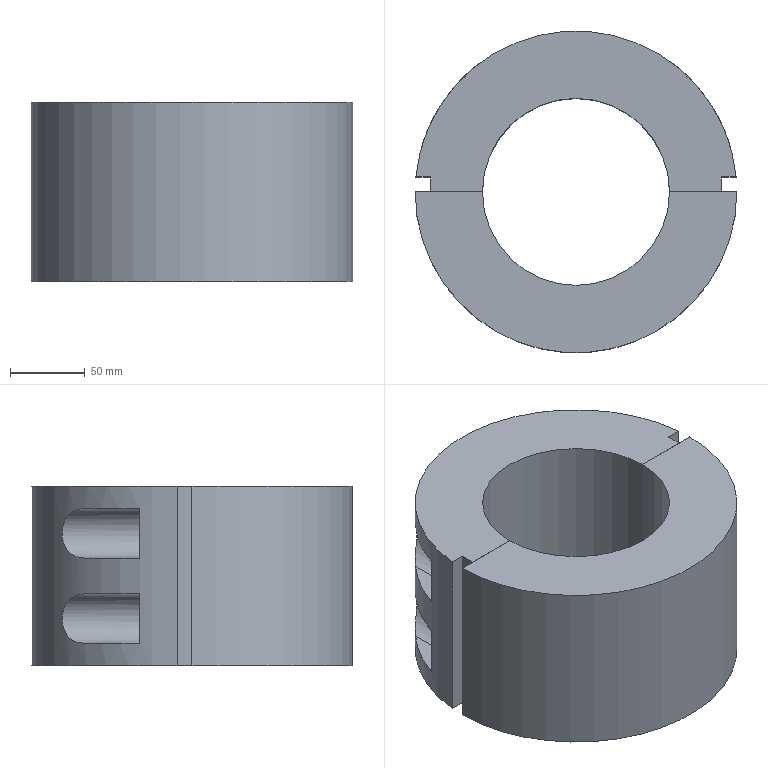Part | 2 solids | 44 faces | box 215 x 215 x 120 mm | volume 2640481 mm3 | plane 28 | cylinder 16 | commonest cylinder face diameters 17.5 x4 21.5 x4 33 x4 125 x2 215 x2
STEP:
#1=CARTESIAN_POINT('',(-80.,-35.,-79.75));
#2=VERTEX_POINT('',#1);
#3=CARTESIAN_POINT('',(-80.,-35.,-88.5));
#4=DIRECTION('',(0.,-1.,0.));
#5=DIRECTION('',(0.,0.,1.));
#6=AXIS2_PLACEMENT_3D('',#3,#4,#5);
#7=CIRCLE('',#6,8.75);
#8=EDGE_CURVE('',#2,#2,#7,.T.);
#9=ORIENTED_EDGE('',*,*,#8,.F.);
#10=EDGE_LOOP('',(#9));
#11=FACE_BOUND('',#10,.T.);
#12=CARTESIAN_POINT('',(-80.,-35.,-88.5));
#13=DIRECTION('',(0.,1.,0.));
#14=DIRECTION('',(0.,0.,1.));
#15=AXIS2_PLACEMENT_3D('',#12,#13,#14);
#16=PLANE('',#15);
#17=ADVANCED_FACE('',(#11),#16,.T.);
#18=ORIENTED_EDGE('',*,*,#8,.T.);
#19=EDGE_LOOP('',(#18));
#20=FACE_BOUND('',#19,.T.);
#21=CARTESIAN_POINT('',(-80.,0.,-79.75));
#22=VERTEX_POINT('',#21);
#23=CARTESIAN_POINT('',(-80.,0.,-88.5));
#24=DIRECTION('',(0.,-1.,0.));
#25=DIRECTION('',(0.,0.,1.));
#26=AXIS2_PLACEMENT_3D('',#23,#24,#25);
#27=CIRCLE('',#26,8.75);
#28=EDGE_CURVE('',#22,#22,#27,.T.);
#29=ORIENTED_EDGE('',*,*,#28,.F.);
#30=EDGE_LOOP('',(#29));
#31=FACE_BOUND('',#30,.T.);
#32=CARTESIAN_POINT('',(-80.,-35.,-88.5));
#33=DIRECTION('',(0.,1.,0.));
#34=DIRECTION('',(0.,0.,1.));
#35=AXIS2_PLACEMENT_3D('',#32,#33,#34);
#36=CYLINDRICAL_SURFACE('',#35,8.75);
#37=ADVANCED_FACE('',(#20,#31),#36,.F.);
#38=CARTESIAN_POINT('',(-80.,-35.,-40.25));
#39=VERTEX_POINT('',#38);
#40=CARTESIAN_POINT('',(-80.,-35.,-31.5));
#41=DIRECTION('',(0.,1.,0.));
#42=DIRECTION('',(0.,0.,-1.));
#43=AXIS2_PLACEMENT_3D('',#40,#41,#42);
#44=CIRCLE('',#43,8.75);
#45=EDGE_CURVE('',#39,#39,#44,.T.);
#46=ORIENTED_EDGE('',*,*,#45,.T.);
#47=EDGE_LOOP('',(#46));
#48=FACE_BOUND('',#47,.T.);
#49=CARTESIAN_POINT('',(-80.,-35.,-31.5));
#50=DIRECTION('',(0.,-1.,0.));
#51=DIRECTION('',(0.,0.,-1.));
#52=AXIS2_PLACEMENT_3D('',#49,#50,#51);
#53=PLANE('',#52);
#54=ADVANCED_FACE('',(#48),#53,.F.);
#55=ORIENTED_EDGE('',*,*,#45,.F.);
#56=EDGE_LOOP('',(#55));
#57=FACE_BOUND('',#56,.T.);
#58=CARTESIAN_POINT('',(-80.,0.,-22.75));
#59=VERTEX_POINT('',#58);
#60=CARTESIAN_POINT('',(-80.,0.,-31.5));
#61=DIRECTION('',(0.,-1.,0.));
#62=DIRECTION('',(0.,0.,1.));
#63=AXIS2_PLACEMENT_3D('',#60,#61,#62);
#64=CIRCLE('',#63,8.75);
#65=EDGE_CURVE('',#59,#59,#64,.T.);
#66=ORIENTED_EDGE('',*,*,#65,.F.);
#67=EDGE_LOOP('',(#66));
#68=FACE_BOUND('',#67,.T.);
#69=CARTESIAN_POINT('',(-80.,-35.,-31.5));
#70=DIRECTION('',(0.,1.,0.));
#71=DIRECTION('',(0.,0.,1.));
#72=AXIS2_PLACEMENT_3D('',#69,#70,#71);
#73=CYLINDRICAL_SURFACE('',#72,8.75);
#74=ADVANCED_FACE('',(#57,#68),#73,.F.);
#75=CARTESIAN_POINT('',(80.,-35.,-79.75));
#76=VERTEX_POINT('',#75);
#77=CARTESIAN_POINT('',(80.,-35.,-88.5));
#78=DIRECTION('',(0.,1.,0.));
#79=DIRECTION('',(0.,0.,1.));
#80=AXIS2_PLACEMENT_3D('',#77,#78,#79);
#81=CIRCLE('',#80,8.75);
#82=EDGE_CURVE('',#76,#76,#81,.F.);
#83=ORIENTED_EDGE('',*,*,#82,.F.);
#84=EDGE_LOOP('',(#83));
#85=FACE_BOUND('',#84,.T.);
#86=CARTESIAN_POINT('',(80.,-35.,-88.5));
#87=DIRECTION('',(0.,1.,0.));
#88=DIRECTION('',(0.,0.,1.));
#89=AXIS2_PLACEMENT_3D('',#86,#87,#88);
#90=PLANE('',#89);
#91=ADVANCED_FACE('',(#85),#90,.T.);
#92=CARTESIAN_POINT('',(80.,-35.,-40.25));
#93=VERTEX_POINT('',#92);
#94=CARTESIAN_POINT('',(80.,-35.,-31.5));
#95=DIRECTION('',(0.,-1.,0.));
#96=DIRECTION('',(0.,0.,-1.));
#97=AXIS2_PLACEMENT_3D('',#94,#95,#96);
#98=CIRCLE('',#97,8.75);
#99=EDGE_CURVE('',#93,#93,#98,.F.);
#100=ORIENTED_EDGE('',*,*,#99,.T.);
#101=EDGE_LOOP('',(#100));
#102=FACE_BOUND('',#101,.T.);
#103=CARTESIAN_POINT('',(80.,-35.,-31.5));
#104=DIRECTION('',(0.,-1.,0.));
#105=DIRECTION('',(0.,0.,-1.));
#106=AXIS2_PLACEMENT_3D('',#103,#104,#105);
#107=PLANE('',#106);
#108=ADVANCED_FACE('',(#102),#107,.F.);
#109=ORIENTED_EDGE('',*,*,#82,.T.);
#110=EDGE_LOOP('',(#109));
#111=FACE_BOUND('',#110,.T.);
#112=CARTESIAN_POINT('',(80.,0.,-79.75));
#113=VERTEX_POINT('',#112);
#114=CARTESIAN_POINT('',(80.,0.,-88.5));
#115=DIRECTION('',(0.,1.,0.));
#116=DIRECTION('',(0.,0.,1.));
#117=AXIS2_PLACEMENT_3D('',#114,#115,#116);
#118=CIRCLE('',#117,8.75);
#119=EDGE_CURVE('',#113,#113,#118,.T.);
#120=ORIENTED_EDGE('',*,*,#119,.T.);
#121=EDGE_LOOP('',(#120));
#122=FACE_BOUND('',#121,.T.);
#123=CARTESIAN_POINT('',(80.,-35.,-88.5));
#124=DIRECTION('',(0.,1.,0.));
#125=DIRECTION('',(0.,0.,1.));
#126=AXIS2_PLACEMENT_3D('',#123,#124,#125);
#127=CYLINDRICAL_SURFACE('',#126,8.75);
#128=ADVANCED_FACE('',(#111,#122),#127,.F.);
#129=ORIENTED_EDGE('',*,*,#99,.F.);
#130=EDGE_LOOP('',(#129));
#131=FACE_BOUND('',#130,.T.);
#132=CARTESIAN_POINT('',(80.,0.,-22.75));
#133=VERTEX_POINT('',#132);
#134=CARTESIAN_POINT('',(80.,0.,-31.5));
#135=DIRECTION('',(0.,1.,0.));
#136=DIRECTION('',(0.,0.,1.));
#137=AXIS2_PLACEMENT_3D('',#134,#135,#136);
#138=CIRCLE('',#137,8.75);
#139=EDGE_CURVE('',#133,#133,#138,.F.);
#140=ORIENTED_EDGE('',*,*,#139,.F.);
#141=EDGE_LOOP('',(#140));
#142=FACE_BOUND('',#141,.T.);
#143=CARTESIAN_POINT('',(80.,-35.,-31.5));
#144=DIRECTION('',(0.,1.,0.));
#145=DIRECTION('',(0.,0.,1.));
#146=AXIS2_PLACEMENT_3D('',#143,#144,#145);
#147=CYLINDRICAL_SURFACE('',#146,8.75);
#148=ADVANCED_FACE('',(#131,#142),#147,.F.);
#149=ORIENTED_EDGE('',*,*,#139,.T.);
#150=EDGE_LOOP('',(#149));
#151=FACE_BOUND('',#150,.T.);
#152=CARTESIAN_POINT('',(107.5,0.,0.));
#153=VERTEX_POINT('',#152);
#154=CARTESIAN_POINT('',(62.5,0.,0.));
#155=VERTEX_POINT('',#154);
#156=CARTESIAN_POINT('',(107.5,0.,0.));
#157=DIRECTION('',(-1.,0.,0.));
#158=VECTOR('',#157,1000.);
#159=LINE('',#156,#158);
#160=EDGE_CURVE('',#153,#155,#159,.T.);
#161=ORIENTED_EDGE('',*,*,#160,.F.);
#162=CARTESIAN_POINT('',(107.5,0.,-120.));
#163=VERTEX_POINT('',#162);
#164=CARTESIAN_POINT('',(107.5,0.,-120.));
#165=DIRECTION('',(0.,0.,1.));
#166=VECTOR('',#165,1000.);
#167=LINE('',#164,#166);
#168=EDGE_CURVE('',#163,#153,#167,.T.);
#169=ORIENTED_EDGE('',*,*,#168,.F.);
#170=CARTESIAN_POINT('',(62.5,0.,-120.));
#171=VERTEX_POINT('',#170);
#172=CARTESIAN_POINT('',(107.5,0.,-120.));
#173=DIRECTION('',(-1.,0.,0.));
#174=VECTOR('',#173,1000.);
#175=LINE('',#172,#174);
#176=EDGE_CURVE('',#163,#171,#175,.T.);
#177=ORIENTED_EDGE('',*,*,#176,.T.);
#178=CARTESIAN_POINT('',(62.5,0.,-120.));
#179=DIRECTION('',(0.,0.,1.));
#180=VECTOR('',#179,1000.);
#181=LINE('',#178,#180);
#182=EDGE_CURVE('',#171,#155,#181,.T.);
#183=ORIENTED_EDGE('',*,*,#182,.T.);
#184=EDGE_LOOP('',(#161,#169,#177,#183));
#185=FACE_BOUND('',#184,.T.);
#186=ORIENTED_EDGE('',*,*,#119,.F.);
#187=EDGE_LOOP('',(#186));
#188=FACE_BOUND('',#187,.T.);
#189=CARTESIAN_POINT('',(107.5,0.,-120.));
#190=DIRECTION('',(0.,1.,0.));
#191=DIRECTION('',(0.,0.,1.));
#192=AXIS2_PLACEMENT_3D('',#189,#190,#191);
#193=PLANE('',#192);
#194=ADVANCED_FACE('',(#151,#185,#188),#193,.T.);
#195=CARTESIAN_POINT('',(-107.5,0.,0.));
#196=VERTEX_POINT('',#195);
#197=CARTESIAN_POINT('',(0.,0.,0.));
#198=DIRECTION('',(0.,0.,1.));
#199=DIRECTION('',(1.,0.,0.));
#200=AXIS2_PLACEMENT_3D('',#197,#198,#199);
#201=CIRCLE('',#200,107.5);
#202=EDGE_CURVE('',#196,#153,#201,.T.);
#203=ORIENTED_EDGE('',*,*,#202,.F.);
#204=CARTESIAN_POINT('',(-107.5,0.,-120.));
#205=VERTEX_POINT('',#204);
#206=CARTESIAN_POINT('',(-107.5,0.,-120.));
#207=DIRECTION('',(0.,0.,1.));
#208=VECTOR('',#207,1000.);
#209=LINE('',#206,#208);
#210=EDGE_CURVE('',#205,#196,#209,.T.);
#211=ORIENTED_EDGE('',*,*,#210,.F.);
#212=CARTESIAN_POINT('',(0.,0.,-120.));
#213=DIRECTION('',(0.,0.,1.));
#214=DIRECTION('',(1.,0.,0.));
#215=AXIS2_PLACEMENT_3D('',#212,#213,#214);
#216=CIRCLE('',#215,107.5);
#217=EDGE_CURVE('',#205,#163,#216,.T.);
#218=ORIENTED_EDGE('',*,*,#217,.T.);
#219=ORIENTED_EDGE('',*,*,#168,.T.);
#220=EDGE_LOOP('',(#203,#211,#218,#219));
#221=FACE_BOUND('',#220,.T.);
#222=CARTESIAN_POINT('',(0.,0.,-120.));
#223=DIRECTION('',(0.,0.,1.));
#224=DIRECTION('',(1.,0.,0.));
#225=AXIS2_PLACEMENT_3D('',#222,#223,#224);
#226=CYLINDRICAL_SURFACE('',#225,107.5);
#227=ADVANCED_FACE('',(#221),#226,.T.);
#228=CARTESIAN_POINT('',(-62.5,0.,-120.));
#229=VERTEX_POINT('',#228);
#230=CARTESIAN_POINT('',(-62.5,0.,-120.));
#231=DIRECTION('',(-1.,0.,0.));
#232=VECTOR('',#231,1000.);
#233=LINE('',#230,#232);
#234=EDGE_CURVE('',#229,#205,#233,.T.);
#235=ORIENTED_EDGE('',*,*,#234,.F.);
#236=CARTESIAN_POINT('',(0.,0.,-120.));
#237=DIRECTION('',(0.,0.,-1.));
#238=DIRECTION('',(1.,0.,0.));
#239=AXIS2_PLACEMENT_3D('',#236,#237,#238);
#240=CIRCLE('',#239,62.5);
#241=EDGE_CURVE('',#171,#229,#240,.T.);
#242=ORIENTED_EDGE('',*,*,#241,.F.);
#243=ORIENTED_EDGE('',*,*,#176,.F.);
#244=ORIENTED_EDGE('',*,*,#217,.F.);
#245=EDGE_LOOP('',(#235,#242,#243,#244));
#246=FACE_BOUND('',#245,.T.);
#247=CARTESIAN_POINT('',(0.,0.,-120.));
#248=DIRECTION('',(0.,0.,1.));
#249=DIRECTION('',(1.,0.,0.));
#250=AXIS2_PLACEMENT_3D('',#247,#248,#249);
#251=PLANE('',#250);
#252=ADVANCED_FACE('',(#246),#251,.F.);
#253=CARTESIAN_POINT('',(-62.5,0.,0.));
#254=VERTEX_POINT('',#253);
#255=CARTESIAN_POINT('',(0.,0.,0.));
#256=DIRECTION('',(0.,0.,-1.));
#257=DIRECTION('',(1.,0.,0.));
#258=AXIS2_PLACEMENT_3D('',#255,#256,#257);
#259=CIRCLE('',#258,62.5);
#260=EDGE_CURVE('',#155,#254,#259,.T.);
#261=ORIENTED_EDGE('',*,*,#260,.F.);
#262=ORIENTED_EDGE('',*,*,#182,.F.);
#263=ORIENTED_EDGE('',*,*,#241,.T.);
#264=CARTESIAN_POINT('',(-62.5,0.,-120.));
#265=DIRECTION('',(0.,0.,1.));
#266=VECTOR('',#265,1000.);
#267=LINE('',#264,#266);
#268=EDGE_CURVE('',#229,#254,#267,.T.);
#269=ORIENTED_EDGE('',*,*,#268,.T.);
#270=EDGE_LOOP('',(#261,#262,#263,#269));
#271=FACE_BOUND('',#270,.T.);
#272=CARTESIAN_POINT('',(0.,0.,-120.));
#273=DIRECTION('',(0.,0.,1.));
#274=DIRECTION('',(1.,0.,0.));
#275=AXIS2_PLACEMENT_3D('',#272,#273,#274);
#276=CYLINDRICAL_SURFACE('',#275,62.5);
#277=ADVANCED_FACE('',(#271),#276,.F.);
#278=CARTESIAN_POINT('',(-62.5,0.,0.));
#279=DIRECTION('',(-1.,0.,0.));
#280=VECTOR('',#279,1000.);
#281=LINE('',#278,#280);
#282=EDGE_CURVE('',#254,#196,#281,.T.);
#283=ORIENTED_EDGE('',*,*,#282,.T.);
#284=ORIENTED_EDGE('',*,*,#202,.T.);
#285=ORIENTED_EDGE('',*,*,#160,.T.);
#286=ORIENTED_EDGE('',*,*,#260,.T.);
#287=EDGE_LOOP('',(#283,#284,#285,#286));
#288=FACE_BOUND('',#287,.T.);
#289=CARTESIAN_POINT('',(0.,0.,0.));
#290=DIRECTION('',(0.,0.,1.));
#291=DIRECTION('',(1.,0.,0.));
#292=AXIS2_PLACEMENT_3D('',#289,#290,#291);
#293=PLANE('',#292);
#294=ADVANCED_FACE('',(#288),#293,.T.);
#295=ORIENTED_EDGE('',*,*,#65,.T.);
#296=EDGE_LOOP('',(#295));
#297=FACE_BOUND('',#296,.T.);
#298=ORIENTED_EDGE('',*,*,#28,.T.);
#299=EDGE_LOOP('',(#298));
#300=FACE_BOUND('',#299,.T.);
#301=ORIENTED_EDGE('',*,*,#282,.F.);
#302=ORIENTED_EDGE('',*,*,#268,.F.);
#303=ORIENTED_EDGE('',*,*,#234,.T.);
#304=ORIENTED_EDGE('',*,*,#210,.T.);
#305=EDGE_LOOP('',(#301,#302,#303,#304));
#306=FACE_BOUND('',#305,.T.);
#307=CARTESIAN_POINT('',(-62.5,0.,-120.));
#308=DIRECTION('',(0.,1.,0.));
#309=DIRECTION('',(0.,0.,1.));
#310=AXIS2_PLACEMENT_3D('',#307,#308,#309);
#311=PLANE('',#310);
#312=ADVANCED_FACE('',(#297,#300,#306),#311,.T.);
#313=CLOSED_SHELL('',(#17,#37,#54,#74,#91,#108,#128,#148,#194,#227,#252,#277,#294,#312));
#314=MANIFOLD_SOLID_BREP('',#313);
#315=CARTESIAN_POINT('',(90.75,0.,-88.5));
#316=VERTEX_POINT('',#315);
#317=CARTESIAN_POINT('',(80.,0.,-88.5));
#318=DIRECTION('',(0.,-1.,0.));
#319=DIRECTION('',(1.,0.,0.));
#320=AXIS2_PLACEMENT_3D('',#317,#318,#319);
#321=CIRCLE('',#320,10.75);
#322=EDGE_CURVE('',#316,#316,#321,.T.);
#323=ORIENTED_EDGE('',*,*,#322,.F.);
#324=EDGE_LOOP('',(#323));
#325=FACE_BOUND('',#324,.T.);
#326=CARTESIAN_POINT('',(90.75,0.,-31.5));
#327=VERTEX_POINT('',#326);
#328=CARTESIAN_POINT('',(80.,0.,-31.5));
#329=DIRECTION('',(0.,-1.,0.));
#330=DIRECTION('',(1.,0.,0.));
#331=AXIS2_PLACEMENT_3D('',#328,#329,#330);
#332=CIRCLE('',#331,10.75);
#333=EDGE_CURVE('',#327,#327,#332,.T.);
#334=ORIENTED_EDGE('',*,*,#333,.F.);
#335=EDGE_LOOP('',(#334));
#336=FACE_BOUND('',#335,.T.);
#337=CARTESIAN_POINT('',(62.5,0.,-120.));
#338=VERTEX_POINT('',#337);
#339=CARTESIAN_POINT('',(97.5,0.,-120.));
#340=VERTEX_POINT('',#339);
#341=CARTESIAN_POINT('',(62.5,0.,-120.));
#342=DIRECTION('',(1.,0.,0.));
#343=VECTOR('',#342,1000.);
#344=LINE('',#341,#343);
#345=EDGE_CURVE('',#338,#340,#344,.T.);
#346=ORIENTED_EDGE('',*,*,#345,.T.);
#347=CARTESIAN_POINT('',(97.5,0.,0.));
#348=VERTEX_POINT('',#347);
#349=CARTESIAN_POINT('',(97.5,0.,-120.));
#350=DIRECTION('',(0.,0.,1.));
#351=VECTOR('',#350,1000.);
#352=LINE('',#349,#351);
#353=EDGE_CURVE('',#340,#348,#352,.T.);
#354=ORIENTED_EDGE('',*,*,#353,.T.);
#355=CARTESIAN_POINT('',(62.5,0.,0.));
#356=VERTEX_POINT('',#355);
#357=CARTESIAN_POINT('',(62.5,0.,0.));
#358=DIRECTION('',(1.,0.,0.));
#359=VECTOR('',#358,1000.);
#360=LINE('',#357,#359);
#361=EDGE_CURVE('',#356,#348,#360,.T.);
#362=ORIENTED_EDGE('',*,*,#361,.F.);
#363=CARTESIAN_POINT('',(62.5,0.,-120.));
#364=DIRECTION('',(0.,0.,1.));
#365=VECTOR('',#364,1000.);
#366=LINE('',#363,#365);
#367=EDGE_CURVE('',#338,#356,#366,.T.);
#368=ORIENTED_EDGE('',*,*,#367,.F.);
#369=EDGE_LOOP('',(#346,#354,#362,#368));
#370=FACE_BOUND('',#369,.T.);
#371=CARTESIAN_POINT('',(62.5,0.,-120.));
#372=DIRECTION('',(0.,-1.,0.));
#373=DIRECTION('',(0.,0.,-1.));
#374=AXIS2_PLACEMENT_3D('',#371,#372,#373);
#375=PLANE('',#374);
#376=ADVANCED_FACE('',(#325,#336,#370),#375,.T.);
#377=CARTESIAN_POINT('',(107.034,10.,-120.));
#378=VERTEX_POINT('',#377);
#379=CARTESIAN_POINT('',(107.034,10.,0.));
#380=VERTEX_POINT('',#379);
#381=CARTESIAN_POINT('',(107.034,10.,-120.));
#382=DIRECTION('',(0.,0.,1.));
#383=VECTOR('',#382,1000.);
#384=LINE('',#381,#383);
#385=EDGE_CURVE('',#378,#380,#384,.T.);
#386=ORIENTED_EDGE('',*,*,#385,.F.);
#387=CARTESIAN_POINT('',(-107.034,10.,-120.));
#388=VERTEX_POINT('',#387);
#389=CARTESIAN_POINT('',(0.,0.,-120.));
#390=DIRECTION('',(0.,0.,1.));
#391=DIRECTION('',(1.,0.,0.));
#392=AXIS2_PLACEMENT_3D('',#389,#390,#391);
#393=CIRCLE('',#392,107.5);
#394=EDGE_CURVE('',#378,#388,#393,.T.);
#395=ORIENTED_EDGE('',*,*,#394,.T.);
#396=CARTESIAN_POINT('',(-107.034,10.,0.));
#397=VERTEX_POINT('',#396);
#398=CARTESIAN_POINT('',(-107.034,10.,-120.));
#399=DIRECTION('',(0.,0.,1.));
#400=VECTOR('',#399,1000.);
#401=LINE('',#398,#400);
#402=EDGE_CURVE('',#388,#397,#401,.T.);
#403=ORIENTED_EDGE('',*,*,#402,.T.);
#404=CARTESIAN_POINT('',(0.,0.,0.));
#405=DIRECTION('',(0.,0.,1.));
#406=DIRECTION('',(1.,0.,0.));
#407=AXIS2_PLACEMENT_3D('',#404,#405,#406);
#408=CIRCLE('',#407,107.5);
#409=EDGE_CURVE('',#380,#397,#408,.T.);
#410=ORIENTED_EDGE('',*,*,#409,.F.);
#411=EDGE_LOOP('',(#386,#395,#403,#410));
#412=FACE_BOUND('',#411,.T.);
#413=CARTESIAN_POINT('',(101.643,35.,-72.));
#414=VERTEX_POINT('',#413);
#415=CARTESIAN_POINT('',(80.,71.807,-72.));
#416=VERTEX_POINT('',#415);
#417=CARTESIAN_POINT('',(0.,0.,-72.));
#418=DIRECTION('',(0.,0.,-1.));
#419=DIRECTION('',(-1.,0.,0.));
#420=AXIS2_PLACEMENT_3D('',#417,#418,#419);
#421=CIRCLE('',#420,107.5);
#422=EDGE_CURVE('',#414,#416,#421,.F.);
#423=ORIENTED_EDGE('',*,*,#422,.T.);
#424=CARTESIAN_POINT('',(80.,71.807,-105.));
#425=VERTEX_POINT('',#424);
#426=CARTESIAN_POINT('',(80.,71.807,-72.));
#427=CARTESIAN_POINT('',(78.278,73.725,-72.));
#428=CARTESIAN_POINT('',(74.76,77.37,-72.52));
#429=CARTESIAN_POINT('',(69.34,82.241,-75.352));
#430=CARTESIAN_POINT('',(64.79,85.815,-80.78));
#431=CARTESIAN_POINT('',(62.866,87.196,-88.423));
#432=CARTESIAN_POINT('',(64.747,85.847,-96.157));
#433=CARTESIAN_POINT('',(69.292,82.28,-101.604));
#434=CARTESIAN_POINT('',(74.685,77.444,-104.462));
#435=CARTESIAN_POINT('',(78.274,73.73,-105.));
#436=CARTESIAN_POINT('',(80.,71.807,-105.));
#437=B_SPLINE_CURVE_WITH_KNOTS('',3,(#426,#427,#428,#429,#430,#431,#432,#433,#434,#435,#436),.UNSPECIFIED.,.F.,.F.,(4,1,1,1,1,1,1,1,4),(0.,0.007628,0.01526,0.02288,0.03051,0.03814,0.04577,0.05339,0.06102),.UNSPECIFIED.);
#438=EDGE_CURVE('',#416,#425,#437,.T.);
#439=ORIENTED_EDGE('',*,*,#438,.T.);
#440=CARTESIAN_POINT('',(101.643,35.,-105.));
#441=VERTEX_POINT('',#440);
#442=CARTESIAN_POINT('',(0.,0.,-105.));
#443=DIRECTION('',(0.,0.,1.));
#444=DIRECTION('',(1.,0.,0.));
#445=AXIS2_PLACEMENT_3D('',#442,#443,#444);
#446=CIRCLE('',#445,107.5);
#447=EDGE_CURVE('',#425,#441,#446,.F.);
#448=ORIENTED_EDGE('',*,*,#447,.T.);
#449=CARTESIAN_POINT('',(101.643,35.,-120.));
#450=DIRECTION('',(0.,0.,1.));
#451=VECTOR('',#450,1000.);
#452=LINE('',#449,#451);
#453=EDGE_CURVE('',#441,#414,#452,.T.);
#454=ORIENTED_EDGE('',*,*,#453,.T.);
#455=EDGE_LOOP('',(#423,#439,#448,#454));
#456=FACE_BOUND('',#455,.T.);
#457=CARTESIAN_POINT('',(101.643,35.,-15.));
#458=VERTEX_POINT('',#457);
#459=CARTESIAN_POINT('',(80.,71.807,-15.));
#460=VERTEX_POINT('',#459);
#461=CARTESIAN_POINT('',(0.,0.,-15.));
#462=DIRECTION('',(0.,0.,-1.));
#463=DIRECTION('',(-1.,0.,0.));
#464=AXIS2_PLACEMENT_3D('',#461,#462,#463);
#465=CIRCLE('',#464,107.5);
#466=EDGE_CURVE('',#458,#460,#465,.F.);
#467=ORIENTED_EDGE('',*,*,#466,.T.);
#468=CARTESIAN_POINT('',(80.,71.807,-48.));
#469=VERTEX_POINT('',#468);
#470=CARTESIAN_POINT('',(80.,71.807,-15.));
#471=CARTESIAN_POINT('',(78.278,73.725,-15.));
#472=CARTESIAN_POINT('',(74.76,77.37,-15.52));
#473=CARTESIAN_POINT('',(69.34,82.241,-18.352));
#474=CARTESIAN_POINT('',(64.79,85.815,-23.78));
#475=CARTESIAN_POINT('',(62.866,87.196,-31.423));
#476=CARTESIAN_POINT('',(64.747,85.847,-39.157));
#477=CARTESIAN_POINT('',(69.292,82.28,-44.604));
#478=CARTESIAN_POINT('',(74.685,77.444,-47.462));
#479=CARTESIAN_POINT('',(78.274,73.73,-48.));
#480=CARTESIAN_POINT('',(80.,71.807,-48.));
#481=B_SPLINE_CURVE_WITH_KNOTS('',3,(#470,#471,#472,#473,#474,#475,#476,#477,#478,#479,#480),.UNSPECIFIED.,.F.,.F.,(4,1,1,1,1,1,1,1,4),(0.,0.007628,0.01526,0.02288,0.03051,0.03814,0.04577,0.05339,0.06102),.UNSPECIFIED.);
#482=EDGE_CURVE('',#460,#469,#481,.T.);
#483=ORIENTED_EDGE('',*,*,#482,.T.);
#484=CARTESIAN_POINT('',(101.643,35.,-48.));
#485=VERTEX_POINT('',#484);
#486=CARTESIAN_POINT('',(0.,0.,-48.));
#487=DIRECTION('',(0.,0.,1.));
#488=DIRECTION('',(1.,0.,0.));
#489=AXIS2_PLACEMENT_3D('',#486,#487,#488);
#490=CIRCLE('',#489,107.5);
#491=EDGE_CURVE('',#469,#485,#490,.F.);
#492=ORIENTED_EDGE('',*,*,#491,.T.);
#493=CARTESIAN_POINT('',(101.643,35.,-120.));
#494=DIRECTION('',(0.,0.,1.));
#495=VECTOR('',#494,1000.);
#496=LINE('',#493,#495);
#497=EDGE_CURVE('',#485,#458,#496,.T.);
#498=ORIENTED_EDGE('',*,*,#497,.T.);
#499=EDGE_LOOP('',(#467,#483,#492,#498));
#500=FACE_BOUND('',#499,.T.);
#501=CARTESIAN_POINT('',(-80.,71.807,-48.));
#502=VERTEX_POINT('',#501);
#503=CARTESIAN_POINT('',(-80.,71.807,-15.));
#504=VERTEX_POINT('',#503);
#505=CARTESIAN_POINT('',(-80.,71.807,-48.));
#506=CARTESIAN_POINT('',(-78.278,73.725,-48.));
#507=CARTESIAN_POINT('',(-74.76,77.37,-47.48));
#508=CARTESIAN_POINT('',(-69.34,82.241,-44.648));
#509=CARTESIAN_POINT('',(-64.79,85.815,-39.22));
#510=CARTESIAN_POINT('',(-62.866,87.196,-31.577));
#511=CARTESIAN_POINT('',(-64.747,85.847,-23.843));
#512=CARTESIAN_POINT('',(-69.292,82.28,-18.396));
#513=CARTESIAN_POINT('',(-74.685,77.444,-15.538));
#514=CARTESIAN_POINT('',(-78.274,73.73,-15.));
#515=CARTESIAN_POINT('',(-80.,71.807,-15.));
#516=B_SPLINE_CURVE_WITH_KNOTS('',3,(#505,#506,#507,#508,#509,#510,#511,#512,#513,#514,#515),.UNSPECIFIED.,.F.,.F.,(4,1,1,1,1,1,1,1,4),(0.,0.007628,0.01526,0.02288,0.03051,0.03814,0.04577,0.05339,0.06102),.UNSPECIFIED.);
#517=EDGE_CURVE('',#502,#504,#516,.T.);
#518=ORIENTED_EDGE('',*,*,#517,.T.);
#519=CARTESIAN_POINT('',(-101.643,35.,-15.));
#520=VERTEX_POINT('',#519);
#521=CARTESIAN_POINT('',(0.,0.,-15.));
#522=DIRECTION('',(0.,0.,-1.));
#523=DIRECTION('',(-1.,0.,0.));
#524=AXIS2_PLACEMENT_3D('',#521,#522,#523);
#525=CIRCLE('',#524,107.5);
#526=EDGE_CURVE('',#504,#520,#525,.F.);
#527=ORIENTED_EDGE('',*,*,#526,.T.);
#528=CARTESIAN_POINT('',(-101.643,35.,-48.));
#529=VERTEX_POINT('',#528);
#530=CARTESIAN_POINT('',(-101.643,35.,-120.));
#531=DIRECTION('',(0.,0.,1.));
#532=VECTOR('',#531,1000.);
#533=LINE('',#530,#532);
#534=EDGE_CURVE('',#520,#529,#533,.F.);
#535=ORIENTED_EDGE('',*,*,#534,.T.);
#536=CARTESIAN_POINT('',(0.,0.,-48.));
#537=DIRECTION('',(0.,0.,1.));
#538=DIRECTION('',(1.,0.,0.));
#539=AXIS2_PLACEMENT_3D('',#536,#537,#538);
#540=CIRCLE('',#539,107.5);
#541=EDGE_CURVE('',#529,#502,#540,.F.);
#542=ORIENTED_EDGE('',*,*,#541,.T.);
#543=EDGE_LOOP('',(#518,#527,#535,#542));
#544=FACE_BOUND('',#543,.T.);
#545=CARTESIAN_POINT('',(-80.,71.807,-105.));
#546=VERTEX_POINT('',#545);
#547=CARTESIAN_POINT('',(-80.,71.807,-72.));
#548=VERTEX_POINT('',#547);
#549=CARTESIAN_POINT('',(-80.,71.807,-105.));
#550=CARTESIAN_POINT('',(-78.278,73.725,-105.));
#551=CARTESIAN_POINT('',(-74.76,77.37,-104.48));
#552=CARTESIAN_POINT('',(-69.34,82.241,-101.648));
#553=CARTESIAN_POINT('',(-64.79,85.815,-96.22));
#554=CARTESIAN_POINT('',(-62.866,87.196,-88.577));
#555=CARTESIAN_POINT('',(-64.747,85.847,-80.843));
#556=CARTESIAN_POINT('',(-69.292,82.28,-75.396));
#557=CARTESIAN_POINT('',(-74.685,77.444,-72.538));
#558=CARTESIAN_POINT('',(-78.274,73.73,-72.));
#559=CARTESIAN_POINT('',(-80.,71.807,-72.));
#560=B_SPLINE_CURVE_WITH_KNOTS('',3,(#549,#550,#551,#552,#553,#554,#555,#556,#557,#558,#559),.UNSPECIFIED.,.F.,.F.,(4,1,1,1,1,1,1,1,4),(0.,0.007628,0.01526,0.02288,0.03051,0.03814,0.04577,0.05339,0.06102),.UNSPECIFIED.);
#561=EDGE_CURVE('',#546,#548,#560,.T.);
#562=ORIENTED_EDGE('',*,*,#561,.T.);
#563=CARTESIAN_POINT('',(-101.643,35.,-72.));
#564=VERTEX_POINT('',#563);
#565=CARTESIAN_POINT('',(0.,0.,-72.));
#566=DIRECTION('',(0.,0.,1.));
#567=DIRECTION('',(1.,0.,0.));
#568=AXIS2_PLACEMENT_3D('',#565,#566,#567);
#569=CIRCLE('',#568,107.5);
#570=EDGE_CURVE('',#548,#564,#569,.T.);
#571=ORIENTED_EDGE('',*,*,#570,.T.);
#572=CARTESIAN_POINT('',(-101.643,35.,-105.));
#573=VERTEX_POINT('',#572);
#574=CARTESIAN_POINT('',(-101.643,35.,-120.));
#575=DIRECTION('',(0.,0.,1.));
#576=VECTOR('',#575,1000.);
#577=LINE('',#574,#576);
#578=EDGE_CURVE('',#564,#573,#577,.F.);
#579=ORIENTED_EDGE('',*,*,#578,.T.);
#580=CARTESIAN_POINT('',(0.,0.,-105.));
#581=DIRECTION('',(0.,0.,1.));
#582=DIRECTION('',(1.,0.,0.));
#583=AXIS2_PLACEMENT_3D('',#580,#581,#582);
#584=CIRCLE('',#583,107.5);
#585=EDGE_CURVE('',#573,#546,#584,.F.);
#586=ORIENTED_EDGE('',*,*,#585,.T.);
#587=EDGE_LOOP('',(#562,#571,#579,#586));
#588=FACE_BOUND('',#587,.T.);
#589=CARTESIAN_POINT('',(0.,0.,-120.));
#590=DIRECTION('',(0.,0.,1.));
#591=DIRECTION('',(1.,0.,0.));
#592=AXIS2_PLACEMENT_3D('',#589,#590,#591);
#593=CYLINDRICAL_SURFACE('',#592,107.5);
#594=ADVANCED_FACE('',(#412,#456,#500,#544,#588),#593,.T.);
#595=CARTESIAN_POINT('',(97.5,10.,-120.));
#596=VERTEX_POINT('',#595);
#597=CARTESIAN_POINT('',(107.034,10.,-120.));
#598=DIRECTION('',(-1.,0.,0.));
#599=VECTOR('',#598,1000.);
#600=LINE('',#597,#599);
#601=EDGE_CURVE('',#378,#596,#600,.T.);
#602=ORIENTED_EDGE('',*,*,#601,.T.);
#603=CARTESIAN_POINT('',(97.5,10.,-120.));
#604=DIRECTION('',(0.,-1.,0.));
#605=VECTOR('',#604,1000.);
#606=LINE('',#603,#605);
#607=EDGE_CURVE('',#596,#340,#606,.T.);
#608=ORIENTED_EDGE('',*,*,#607,.T.);
#609=ORIENTED_EDGE('',*,*,#345,.F.);
#610=CARTESIAN_POINT('',(-62.5,0.,-120.));
#611=VERTEX_POINT('',#610);
#612=CARTESIAN_POINT('',(0.,0.,-120.));
#613=DIRECTION('',(0.,0.,-1.));
#614=DIRECTION('',(1.,0.,0.));
#615=AXIS2_PLACEMENT_3D('',#612,#613,#614);
#616=CIRCLE('',#615,62.5);
#617=EDGE_CURVE('',#611,#338,#616,.T.);
#618=ORIENTED_EDGE('',*,*,#617,.F.);
#619=CARTESIAN_POINT('',(-97.5,0.,-120.));
#620=VERTEX_POINT('',#619);
#621=CARTESIAN_POINT('',(-107.5,0.,-120.));
#622=DIRECTION('',(1.,0.,0.));
#623=VECTOR('',#622,1000.);
#624=LINE('',#621,#623);
#625=EDGE_CURVE('',#620,#611,#624,.T.);
#626=ORIENTED_EDGE('',*,*,#625,.F.);
#627=CARTESIAN_POINT('',(-97.5,10.,-120.));
#628=VERTEX_POINT('',#627);
#629=CARTESIAN_POINT('',(-97.5,0.,-120.));
#630=DIRECTION('',(0.,1.,0.));
#631=VECTOR('',#630,1000.);
#632=LINE('',#629,#631);
#633=EDGE_CURVE('',#620,#628,#632,.T.);
#634=ORIENTED_EDGE('',*,*,#633,.T.);
#635=CARTESIAN_POINT('',(-97.5,10.,-120.));
#636=DIRECTION('',(-1.,0.,0.));
#637=VECTOR('',#636,1000.);
#638=LINE('',#635,#637);
#639=EDGE_CURVE('',#628,#388,#638,.T.);
#640=ORIENTED_EDGE('',*,*,#639,.T.);
#641=ORIENTED_EDGE('',*,*,#394,.F.);
#642=EDGE_LOOP('',(#602,#608,#609,#618,#626,#634,#640,#641));
#643=FACE_BOUND('',#642,.T.);
#644=CARTESIAN_POINT('',(0.,0.,-120.));
#645=DIRECTION('',(0.,0.,-1.));
#646=DIRECTION('',(-1.,0.,0.));
#647=AXIS2_PLACEMENT_3D('',#644,#645,#646);
#648=PLANE('',#647);
#649=ADVANCED_FACE('',(#643),#648,.T.);
#650=CARTESIAN_POINT('',(97.5,10.,0.));
#651=VERTEX_POINT('',#650);
#652=CARTESIAN_POINT('',(97.5,10.,0.));
#653=DIRECTION('',(0.,-1.,0.));
#654=VECTOR('',#653,1000.);
#655=LINE('',#652,#654);
#656=EDGE_CURVE('',#651,#348,#655,.T.);
#657=ORIENTED_EDGE('',*,*,#656,.F.);
#658=CARTESIAN_POINT('',(107.034,10.,0.));
#659=DIRECTION('',(-1.,0.,0.));
#660=VECTOR('',#659,1000.);
#661=LINE('',#658,#660);
#662=EDGE_CURVE('',#380,#651,#661,.T.);
#663=ORIENTED_EDGE('',*,*,#662,.F.);
#664=ORIENTED_EDGE('',*,*,#409,.T.);
#665=CARTESIAN_POINT('',(-97.5,10.,0.));
#666=VERTEX_POINT('',#665);
#667=CARTESIAN_POINT('',(-97.5,10.,0.));
#668=DIRECTION('',(-1.,0.,0.));
#669=VECTOR('',#668,1000.);
#670=LINE('',#667,#669);
#671=EDGE_CURVE('',#666,#397,#670,.T.);
#672=ORIENTED_EDGE('',*,*,#671,.F.);
#673=CARTESIAN_POINT('',(-97.5,0.,0.));
#674=VERTEX_POINT('',#673);
#675=CARTESIAN_POINT('',(-97.5,0.,0.));
#676=DIRECTION('',(0.,1.,0.));
#677=VECTOR('',#676,1000.);
#678=LINE('',#675,#677);
#679=EDGE_CURVE('',#674,#666,#678,.T.);
#680=ORIENTED_EDGE('',*,*,#679,.F.);
#681=CARTESIAN_POINT('',(-62.5,0.,0.));
#682=VERTEX_POINT('',#681);
#683=CARTESIAN_POINT('',(-107.5,0.,0.));
#684=DIRECTION('',(1.,0.,0.));
#685=VECTOR('',#684,1000.);
#686=LINE('',#683,#685);
#687=EDGE_CURVE('',#674,#682,#686,.T.);
#688=ORIENTED_EDGE('',*,*,#687,.T.);
#689=CARTESIAN_POINT('',(0.,0.,0.));
#690=DIRECTION('',(0.,0.,-1.));
#691=DIRECTION('',(1.,0.,0.));
#692=AXIS2_PLACEMENT_3D('',#689,#690,#691);
#693=CIRCLE('',#692,62.5);
#694=EDGE_CURVE('',#682,#356,#693,.T.);
#695=ORIENTED_EDGE('',*,*,#694,.T.);
#696=ORIENTED_EDGE('',*,*,#361,.T.);
#697=EDGE_LOOP('',(#657,#663,#664,#672,#680,#688,#695,#696));
#698=FACE_BOUND('',#697,.T.);
#699=CARTESIAN_POINT('',(0.,0.,0.));
#700=DIRECTION('',(0.,0.,-1.));
#701=DIRECTION('',(-1.,0.,0.));
#702=AXIS2_PLACEMENT_3D('',#699,#700,#701);
#703=PLANE('',#702);
#704=ADVANCED_FACE('',(#698),#703,.F.);
#705=CARTESIAN_POINT('',(-90.75,0.,-88.5));
#706=VERTEX_POINT('',#705);
#707=CARTESIAN_POINT('',(-80.,0.,-88.5));
#708=DIRECTION('',(0.,1.,0.));
#709=DIRECTION('',(-1.,0.,0.));
#710=AXIS2_PLACEMENT_3D('',#707,#708,#709);
#711=CIRCLE('',#710,10.75);
#712=EDGE_CURVE('',#706,#706,#711,.T.);
#713=ORIENTED_EDGE('',*,*,#712,.F.);
#714=EDGE_LOOP('',(#713));
#715=FACE_BOUND('',#714,.T.);
#716=CARTESIAN_POINT('',(-90.75,35.,-88.5));
#717=VERTEX_POINT('',#716);
#718=CARTESIAN_POINT('',(-80.,35.,-88.5));
#719=DIRECTION('',(0.,-1.,0.));
#720=DIRECTION('',(-1.,0.,0.));
#721=AXIS2_PLACEMENT_3D('',#718,#719,#720);
#722=CIRCLE('',#721,10.75);
#723=EDGE_CURVE('',#717,#717,#722,.F.);
#724=ORIENTED_EDGE('',*,*,#723,.T.);
#725=EDGE_LOOP('',(#724));
#726=FACE_BOUND('',#725,.T.);
#727=CARTESIAN_POINT('',(-80.,120.,-88.5));
#728=DIRECTION('',(0.,-1.,0.));
#729=DIRECTION('',(0.,0.,-1.));
#730=AXIS2_PLACEMENT_3D('',#727,#728,#729);
#731=CYLINDRICAL_SURFACE('',#730,10.75);
#732=ADVANCED_FACE('',(#715,#726),#731,.F.);
#733=CARTESIAN_POINT('',(-80.,35.,-72.));
#734=VERTEX_POINT('',#733);
#735=CARTESIAN_POINT('',(-80.,120.,-72.));
#736=DIRECTION('',(0.,-1.,0.));
#737=VECTOR('',#736,1000.);
#738=LINE('',#735,#737);
#739=EDGE_CURVE('',#548,#734,#738,.T.);
#740=ORIENTED_EDGE('',*,*,#739,.F.);
#741=ORIENTED_EDGE('',*,*,#561,.F.);
#742=CARTESIAN_POINT('',(-80.,35.,-105.));
#743=VERTEX_POINT('',#742);
#744=CARTESIAN_POINT('',(-80.,120.,-105.));
#745=DIRECTION('',(0.,-1.,0.));
#746=VECTOR('',#745,1000.);
#747=LINE('',#744,#746);
#748=EDGE_CURVE('',#546,#743,#747,.T.);
#749=ORIENTED_EDGE('',*,*,#748,.T.);
#750=CARTESIAN_POINT('',(-80.,35.,-88.5));
#751=DIRECTION('',(0.,-1.,0.));
#752=DIRECTION('',(-1.,0.,0.));
#753=AXIS2_PLACEMENT_3D('',#750,#751,#752);
#754=CIRCLE('',#753,16.5);
#755=EDGE_CURVE('',#743,#734,#754,.T.);
#756=ORIENTED_EDGE('',*,*,#755,.T.);
#757=EDGE_LOOP('',(#740,#741,#749,#756));
#758=FACE_BOUND('',#757,.T.);
#759=CARTESIAN_POINT('',(-80.,120.,-88.5));
#760=DIRECTION('',(0.,-1.,0.));
#761=DIRECTION('',(0.,0.,-1.));
#762=AXIS2_PLACEMENT_3D('',#759,#760,#761);
#763=CYLINDRICAL_SURFACE('',#762,16.5);
#764=ADVANCED_FACE('',(#758),#763,.F.);
#765=CARTESIAN_POINT('',(-107.5,35.,-105.));
#766=DIRECTION('',(1.,0.,0.));
#767=VECTOR('',#766,1000.);
#768=LINE('',#765,#767);
#769=EDGE_CURVE('',#573,#743,#768,.T.);
#770=ORIENTED_EDGE('',*,*,#769,.F.);
#771=ORIENTED_EDGE('',*,*,#578,.F.);
#772=CARTESIAN_POINT('',(-80.,35.,-72.));
#773=DIRECTION('',(-1.,0.,0.));
#774=VECTOR('',#773,1000.);
#775=LINE('',#772,#774);
#776=EDGE_CURVE('',#734,#564,#775,.T.);
#777=ORIENTED_EDGE('',*,*,#776,.F.);
#778=ORIENTED_EDGE('',*,*,#755,.F.);
#779=EDGE_LOOP('',(#770,#771,#777,#778));
#780=FACE_BOUND('',#779,.T.);
#781=ORIENTED_EDGE('',*,*,#723,.F.);
#782=EDGE_LOOP('',(#781));
#783=FACE_BOUND('',#782,.T.);
#784=CARTESIAN_POINT('',(-80.,35.,-88.5));
#785=DIRECTION('',(0.,1.,0.));
#786=DIRECTION('',(0.,0.,1.));
#787=AXIS2_PLACEMENT_3D('',#784,#785,#786);
#788=PLANE('',#787);
#789=ADVANCED_FACE('',(#780,#783),#788,.T.);
#790=ORIENTED_EDGE('',*,*,#776,.T.);
#791=ORIENTED_EDGE('',*,*,#570,.F.);
#792=ORIENTED_EDGE('',*,*,#739,.T.);
#793=EDGE_LOOP('',(#790,#791,#792));
#794=FACE_BOUND('',#793,.T.);
#795=CARTESIAN_POINT('',(-80.,120.,-72.));
#796=DIRECTION('',(0.,0.,-1.));
#797=DIRECTION('',(1.,0.,0.));
#798=AXIS2_PLACEMENT_3D('',#795,#796,#797);
#799=PLANE('',#798);
#800=ADVANCED_FACE('',(#794),#799,.T.);
#801=ORIENTED_EDGE('',*,*,#748,.F.);
#802=ORIENTED_EDGE('',*,*,#585,.F.);
#803=ORIENTED_EDGE('',*,*,#769,.T.);
#804=EDGE_LOOP('',(#801,#802,#803));
#805=FACE_BOUND('',#804,.T.);
#806=CARTESIAN_POINT('',(-107.5,120.,-105.));
#807=DIRECTION('',(0.,0.,1.));
#808=DIRECTION('',(-1.,0.,0.));
#809=AXIS2_PLACEMENT_3D('',#806,#807,#808);
#810=PLANE('',#809);
#811=ADVANCED_FACE('',(#805),#810,.T.);
#812=CARTESIAN_POINT('',(-80.,35.,-15.));
#813=VERTEX_POINT('',#812);
#814=CARTESIAN_POINT('',(-80.,35.,-15.));
#815=DIRECTION('',(-1.,0.,0.));
#816=VECTOR('',#815,1000.);
#817=LINE('',#814,#816);
#818=EDGE_CURVE('',#813,#520,#817,.T.);
#819=ORIENTED_EDGE('',*,*,#818,.T.);
#820=ORIENTED_EDGE('',*,*,#526,.F.);
#821=CARTESIAN_POINT('',(-80.,120.,-15.));
#822=DIRECTION('',(0.,-1.,0.));
#823=VECTOR('',#822,1000.);
#824=LINE('',#821,#823);
#825=EDGE_CURVE('',#504,#813,#824,.T.);
#826=ORIENTED_EDGE('',*,*,#825,.T.);
#827=EDGE_LOOP('',(#819,#820,#826));
#828=FACE_BOUND('',#827,.T.);
#829=CARTESIAN_POINT('',(-80.,120.,-15.));
#830=DIRECTION('',(0.,0.,-1.));
#831=DIRECTION('',(1.,0.,0.));
#832=AXIS2_PLACEMENT_3D('',#829,#830,#831);
#833=PLANE('',#832);
#834=ADVANCED_FACE('',(#828),#833,.T.);
#835=CARTESIAN_POINT('',(-80.,35.,-48.));
#836=VERTEX_POINT('',#835);
#837=CARTESIAN_POINT('',(-107.5,35.,-48.));
#838=DIRECTION('',(1.,0.,0.));
#839=VECTOR('',#838,1000.);
#840=LINE('',#837,#839);
#841=EDGE_CURVE('',#529,#836,#840,.T.);
#842=ORIENTED_EDGE('',*,*,#841,.F.);
#843=ORIENTED_EDGE('',*,*,#534,.F.);
#844=ORIENTED_EDGE('',*,*,#818,.F.);
#845=CARTESIAN_POINT('',(-80.,35.,-31.5));
#846=DIRECTION('',(0.,-1.,0.));
#847=DIRECTION('',(-1.,0.,0.));
#848=AXIS2_PLACEMENT_3D('',#845,#846,#847);
#849=CIRCLE('',#848,16.5);
#850=EDGE_CURVE('',#836,#813,#849,.T.);
#851=ORIENTED_EDGE('',*,*,#850,.F.);
#852=EDGE_LOOP('',(#842,#843,#844,#851));
#853=FACE_BOUND('',#852,.T.);
#854=CARTESIAN_POINT('',(-90.75,35.,-31.5));
#855=VERTEX_POINT('',#854);
#856=CARTESIAN_POINT('',(-80.,35.,-31.5));
#857=DIRECTION('',(0.,-1.,0.));
#858=DIRECTION('',(-1.,0.,0.));
#859=AXIS2_PLACEMENT_3D('',#856,#857,#858);
#860=CIRCLE('',#859,10.75);
#861=EDGE_CURVE('',#855,#855,#860,.F.);
#862=ORIENTED_EDGE('',*,*,#861,.F.);
#863=EDGE_LOOP('',(#862));
#864=FACE_BOUND('',#863,.T.);
#865=CARTESIAN_POINT('',(-80.,35.,-31.5));
#866=DIRECTION('',(0.,1.,0.));
#867=DIRECTION('',(0.,0.,1.));
#868=AXIS2_PLACEMENT_3D('',#865,#866,#867);
#869=PLANE('',#868);
#870=ADVANCED_FACE('',(#853,#864),#869,.T.);
#871=CARTESIAN_POINT('',(-80.,120.,-48.));
#872=DIRECTION('',(0.,-1.,0.));
#873=VECTOR('',#872,1000.);
#874=LINE('',#871,#873);
#875=EDGE_CURVE('',#502,#836,#874,.T.);
#876=ORIENTED_EDGE('',*,*,#875,.F.);
#877=ORIENTED_EDGE('',*,*,#541,.F.);
#878=ORIENTED_EDGE('',*,*,#841,.T.);
#879=EDGE_LOOP('',(#876,#877,#878));
#880=FACE_BOUND('',#879,.T.);
#881=CARTESIAN_POINT('',(-107.5,120.,-48.));
#882=DIRECTION('',(0.,0.,1.));
#883=DIRECTION('',(-1.,0.,0.));
#884=AXIS2_PLACEMENT_3D('',#881,#882,#883);
#885=PLANE('',#884);
#886=ADVANCED_FACE('',(#880),#885,.T.);
#887=ORIENTED_EDGE('',*,*,#825,.F.);
#888=ORIENTED_EDGE('',*,*,#517,.F.);
#889=ORIENTED_EDGE('',*,*,#875,.T.);
#890=ORIENTED_EDGE('',*,*,#850,.T.);
#891=EDGE_LOOP('',(#887,#888,#889,#890));
#892=FACE_BOUND('',#891,.T.);
#893=CARTESIAN_POINT('',(-80.,120.,-31.5));
#894=DIRECTION('',(0.,-1.,0.));
#895=DIRECTION('',(0.,0.,-1.));
#896=AXIS2_PLACEMENT_3D('',#893,#894,#895);
#897=CYLINDRICAL_SURFACE('',#896,16.5);
#898=ADVANCED_FACE('',(#892),#897,.F.);
#899=CARTESIAN_POINT('',(-90.75,0.,-31.5));
#900=VERTEX_POINT('',#899);
#901=CARTESIAN_POINT('',(-80.,0.,-31.5));
#902=DIRECTION('',(0.,1.,0.));
#903=DIRECTION('',(-1.,0.,0.));
#904=AXIS2_PLACEMENT_3D('',#901,#902,#903);
#905=CIRCLE('',#904,10.75);
#906=EDGE_CURVE('',#900,#900,#905,.T.);
#907=ORIENTED_EDGE('',*,*,#906,.F.);
#908=EDGE_LOOP('',(#907));
#909=FACE_BOUND('',#908,.T.);
#910=ORIENTED_EDGE('',*,*,#861,.T.);
#911=EDGE_LOOP('',(#910));
#912=FACE_BOUND('',#911,.T.);
#913=CARTESIAN_POINT('',(-80.,120.,-31.5));
#914=DIRECTION('',(0.,-1.,0.));
#915=DIRECTION('',(0.,0.,-1.));
#916=AXIS2_PLACEMENT_3D('',#913,#914,#915);
#917=CYLINDRICAL_SURFACE('',#916,10.75);
#918=ADVANCED_FACE('',(#909,#912),#917,.F.);
#919=ORIENTED_EDGE('',*,*,#333,.T.);
#920=EDGE_LOOP('',(#919));
#921=FACE_BOUND('',#920,.T.);
#922=CARTESIAN_POINT('',(90.75,35.,-31.5));
#923=VERTEX_POINT('',#922);
#924=CARTESIAN_POINT('',(80.,35.,-31.5));
#925=DIRECTION('',(0.,1.,0.));
#926=DIRECTION('',(1.,0.,0.));
#927=AXIS2_PLACEMENT_3D('',#924,#925,#926);
#928=CIRCLE('',#927,10.75);
#929=EDGE_CURVE('',#923,#923,#928,.T.);
#930=ORIENTED_EDGE('',*,*,#929,.T.);
#931=EDGE_LOOP('',(#930));
#932=FACE_BOUND('',#931,.T.);
#933=CARTESIAN_POINT('',(80.,120.,-31.5));
#934=DIRECTION('',(0.,-1.,0.));
#935=DIRECTION('',(0.,0.,-1.));
#936=AXIS2_PLACEMENT_3D('',#933,#934,#935);
#937=CYLINDRICAL_SURFACE('',#936,10.75);
#938=ADVANCED_FACE('',(#921,#932),#937,.F.);
#939=ORIENTED_EDGE('',*,*,#322,.T.);
#940=EDGE_LOOP('',(#939));
#941=FACE_BOUND('',#940,.T.);
#942=CARTESIAN_POINT('',(90.75,35.,-88.5));
#943=VERTEX_POINT('',#942);
#944=CARTESIAN_POINT('',(80.,35.,-88.5));
#945=DIRECTION('',(0.,1.,0.));
#946=DIRECTION('',(1.,0.,0.));
#947=AXIS2_PLACEMENT_3D('',#944,#945,#946);
#948=CIRCLE('',#947,10.75);
#949=EDGE_CURVE('',#943,#943,#948,.T.);
#950=ORIENTED_EDGE('',*,*,#949,.T.);
#951=EDGE_LOOP('',(#950));
#952=FACE_BOUND('',#951,.T.);
#953=CARTESIAN_POINT('',(80.,120.,-88.5));
#954=DIRECTION('',(0.,-1.,0.));
#955=DIRECTION('',(0.,0.,-1.));
#956=AXIS2_PLACEMENT_3D('',#953,#954,#955);
#957=CYLINDRICAL_SURFACE('',#956,10.75);
#958=ADVANCED_FACE('',(#941,#952),#957,.F.);
#959=ORIENTED_EDGE('',*,*,#694,.F.);
#960=CARTESIAN_POINT('',(-62.5,0.,-120.));
#961=DIRECTION('',(0.,0.,1.));
#962=VECTOR('',#961,1000.);
#963=LINE('',#960,#962);
#964=EDGE_CURVE('',#611,#682,#963,.T.);
#965=ORIENTED_EDGE('',*,*,#964,.F.);
#966=ORIENTED_EDGE('',*,*,#617,.T.);
#967=ORIENTED_EDGE('',*,*,#367,.T.);
#968=EDGE_LOOP('',(#959,#965,#966,#967));
#969=FACE_BOUND('',#968,.T.);
#970=CARTESIAN_POINT('',(0.,0.,-120.));
#971=DIRECTION('',(0.,0.,1.));
#972=DIRECTION('',(1.,0.,0.));
#973=AXIS2_PLACEMENT_3D('',#970,#971,#972);
#974=CYLINDRICAL_SURFACE('',#973,62.5);
#975=ADVANCED_FACE('',(#969),#974,.F.);
#976=CARTESIAN_POINT('',(80.,35.,-48.));
#977=VERTEX_POINT('',#976);
#978=CARTESIAN_POINT('',(107.5,35.,-48.));
#979=DIRECTION('',(-1.,0.,0.));
#980=VECTOR('',#979,1000.);
#981=LINE('',#978,#980);
#982=EDGE_CURVE('',#977,#485,#981,.F.);
#983=ORIENTED_EDGE('',*,*,#982,.F.);
#984=CARTESIAN_POINT('',(80.,35.,-15.));
#985=VERTEX_POINT('',#984);
#986=CARTESIAN_POINT('',(80.,35.,-31.5));
#987=DIRECTION('',(0.,1.,0.));
#988=DIRECTION('',(1.,0.,0.));
#989=AXIS2_PLACEMENT_3D('',#986,#987,#988);
#990=CIRCLE('',#989,16.5);
#991=EDGE_CURVE('',#985,#977,#990,.F.);
#992=ORIENTED_EDGE('',*,*,#991,.F.);
#993=CARTESIAN_POINT('',(80.,35.,-15.));
#994=DIRECTION('',(1.,0.,0.));
#995=VECTOR('',#994,1000.);
#996=LINE('',#993,#995);
#997=EDGE_CURVE('',#458,#985,#996,.F.);
#998=ORIENTED_EDGE('',*,*,#997,.F.);
#999=ORIENTED_EDGE('',*,*,#497,.F.);
#1000=EDGE_LOOP('',(#983,#992,#998,#999));
#1001=FACE_BOUND('',#1000,.T.);
#1002=ORIENTED_EDGE('',*,*,#929,.F.);
#1003=EDGE_LOOP('',(#1002));
#1004=FACE_BOUND('',#1003,.T.);
#1005=CARTESIAN_POINT('',(80.,35.,-31.5));
#1006=DIRECTION('',(0.,1.,0.));
#1007=DIRECTION('',(0.,0.,1.));
#1008=AXIS2_PLACEMENT_3D('',#1005,#1006,#1007);
#1009=PLANE('',#1008);
#1010=ADVANCED_FACE('',(#1001,#1004),#1009,.T.);
#1011=CARTESIAN_POINT('',(80.,120.,-48.));
#1012=DIRECTION('',(0.,-1.,0.));
#1013=VECTOR('',#1012,1000.);
#1014=LINE('',#1011,#1013);
#1015=EDGE_CURVE('',#977,#469,#1014,.F.);
#1016=ORIENTED_EDGE('',*,*,#1015,.F.);
#1017=ORIENTED_EDGE('',*,*,#982,.T.);
#1018=ORIENTED_EDGE('',*,*,#491,.F.);
#1019=EDGE_LOOP('',(#1016,#1017,#1018));
#1020=FACE_BOUND('',#1019,.T.);
#1021=CARTESIAN_POINT('',(107.5,120.,-48.));
#1022=DIRECTION('',(0.,0.,1.));
#1023=DIRECTION('',(1.,0.,0.));
#1024=AXIS2_PLACEMENT_3D('',#1021,#1022,#1023);
#1025=PLANE('',#1024);
#1026=ADVANCED_FACE('',(#1020),#1025,.T.);
#1027=CARTESIAN_POINT('',(80.,120.,-15.));
#1028=DIRECTION('',(0.,-1.,0.));
#1029=VECTOR('',#1028,1000.);
#1030=LINE('',#1027,#1029);
#1031=EDGE_CURVE('',#985,#460,#1030,.F.);
#1032=ORIENTED_EDGE('',*,*,#1031,.F.);
#1033=ORIENTED_EDGE('',*,*,#991,.T.);
#1034=ORIENTED_EDGE('',*,*,#1015,.T.);
#1035=ORIENTED_EDGE('',*,*,#482,.F.);
#1036=EDGE_LOOP('',(#1032,#1033,#1034,#1035));
#1037=FACE_BOUND('',#1036,.T.);
#1038=CARTESIAN_POINT('',(80.,120.,-31.5));
#1039=DIRECTION('',(0.,-1.,0.));
#1040=DIRECTION('',(0.,0.,-1.));
#1041=AXIS2_PLACEMENT_3D('',#1038,#1039,#1040);
#1042=CYLINDRICAL_SURFACE('',#1041,16.5);
#1043=ADVANCED_FACE('',(#1037),#1042,.F.);
#1044=ORIENTED_EDGE('',*,*,#997,.T.);
#1045=ORIENTED_EDGE('',*,*,#1031,.T.);
#1046=ORIENTED_EDGE('',*,*,#466,.F.);
#1047=EDGE_LOOP('',(#1044,#1045,#1046));
#1048=FACE_BOUND('',#1047,.T.);
#1049=CARTESIAN_POINT('',(80.,120.,-15.));
#1050=DIRECTION('',(0.,0.,-1.));
#1051=DIRECTION('',(-1.,0.,0.));
#1052=AXIS2_PLACEMENT_3D('',#1049,#1050,#1051);
#1053=PLANE('',#1052);
#1054=ADVANCED_FACE('',(#1048),#1053,.T.);
#1055=CARTESIAN_POINT('',(-97.5,0.,-120.));
#1056=DIRECTION('',(0.,0.,1.));
#1057=VECTOR('',#1056,1000.);
#1058=LINE('',#1055,#1057);
#1059=EDGE_CURVE('',#620,#674,#1058,.T.);
#1060=ORIENTED_EDGE('',*,*,#1059,.F.);
#1061=ORIENTED_EDGE('',*,*,#625,.T.);
#1062=ORIENTED_EDGE('',*,*,#964,.T.);
#1063=ORIENTED_EDGE('',*,*,#687,.F.);
#1064=EDGE_LOOP('',(#1060,#1061,#1062,#1063));
#1065=FACE_BOUND('',#1064,.T.);
#1066=ORIENTED_EDGE('',*,*,#712,.T.);
#1067=EDGE_LOOP('',(#1066));
#1068=FACE_BOUND('',#1067,.T.);
#1069=ORIENTED_EDGE('',*,*,#906,.T.);
#1070=EDGE_LOOP('',(#1069));
#1071=FACE_BOUND('',#1070,.T.);
#1072=CARTESIAN_POINT('',(-107.5,0.,-120.));
#1073=DIRECTION('',(0.,-1.,0.));
#1074=DIRECTION('',(0.,0.,-1.));
#1075=AXIS2_PLACEMENT_3D('',#1072,#1073,#1074);
#1076=PLANE('',#1075);
#1077=ADVANCED_FACE('',(#1065,#1068,#1071),#1076,.T.);
#1078=CARTESIAN_POINT('',(80.,35.,-105.));
#1079=VERTEX_POINT('',#1078);
#1080=CARTESIAN_POINT('',(107.5,35.,-105.));
#1081=DIRECTION('',(-1.,0.,0.));
#1082=VECTOR('',#1081,1000.);
#1083=LINE('',#1080,#1082);
#1084=EDGE_CURVE('',#1079,#441,#1083,.F.);
#1085=ORIENTED_EDGE('',*,*,#1084,.F.);
#1086=CARTESIAN_POINT('',(80.,35.,-72.));
#1087=VERTEX_POINT('',#1086);
#1088=CARTESIAN_POINT('',(80.,35.,-88.5));
#1089=DIRECTION('',(0.,1.,0.));
#1090=DIRECTION('',(1.,0.,0.));
#1091=AXIS2_PLACEMENT_3D('',#1088,#1089,#1090);
#1092=CIRCLE('',#1091,16.5);
#1093=EDGE_CURVE('',#1087,#1079,#1092,.F.);
#1094=ORIENTED_EDGE('',*,*,#1093,.F.);
#1095=CARTESIAN_POINT('',(80.,35.,-72.));
#1096=DIRECTION('',(1.,0.,0.));
#1097=VECTOR('',#1096,1000.);
#1098=LINE('',#1095,#1097);
#1099=EDGE_CURVE('',#414,#1087,#1098,.F.);
#1100=ORIENTED_EDGE('',*,*,#1099,.F.);
#1101=ORIENTED_EDGE('',*,*,#453,.F.);
#1102=EDGE_LOOP('',(#1085,#1094,#1100,#1101));
#1103=FACE_BOUND('',#1102,.T.);
#1104=ORIENTED_EDGE('',*,*,#949,.F.);
#1105=EDGE_LOOP('',(#1104));
#1106=FACE_BOUND('',#1105,.T.);
#1107=CARTESIAN_POINT('',(80.,35.,-88.5));
#1108=DIRECTION('',(0.,1.,0.));
#1109=DIRECTION('',(0.,0.,1.));
#1110=AXIS2_PLACEMENT_3D('',#1107,#1108,#1109);
#1111=PLANE('',#1110);
#1112=ADVANCED_FACE('',(#1103,#1106),#1111,.T.);
#1113=CARTESIAN_POINT('',(80.,120.,-105.));
#1114=DIRECTION('',(0.,-1.,0.));
#1115=VECTOR('',#1114,1000.);
#1116=LINE('',#1113,#1115);
#1117=EDGE_CURVE('',#1079,#425,#1116,.F.);
#1118=ORIENTED_EDGE('',*,*,#1117,.F.);
#1119=ORIENTED_EDGE('',*,*,#1084,.T.);
#1120=ORIENTED_EDGE('',*,*,#447,.F.);
#1121=EDGE_LOOP('',(#1118,#1119,#1120));
#1122=FACE_BOUND('',#1121,.T.);
#1123=CARTESIAN_POINT('',(107.5,120.,-105.));
#1124=DIRECTION('',(0.,0.,1.));
#1125=DIRECTION('',(1.,0.,0.));
#1126=AXIS2_PLACEMENT_3D('',#1123,#1124,#1125);
#1127=PLANE('',#1126);
#1128=ADVANCED_FACE('',(#1122),#1127,.T.);
#1129=CARTESIAN_POINT('',(80.,120.,-72.));
#1130=DIRECTION('',(0.,-1.,0.));
#1131=VECTOR('',#1130,1000.);
#1132=LINE('',#1129,#1131);
#1133=EDGE_CURVE('',#1087,#416,#1132,.F.);
#1134=ORIENTED_EDGE('',*,*,#1133,.F.);
#1135=ORIENTED_EDGE('',*,*,#1093,.T.);
#1136=ORIENTED_EDGE('',*,*,#1117,.T.);
#1137=ORIENTED_EDGE('',*,*,#438,.F.);
#1138=EDGE_LOOP('',(#1134,#1135,#1136,#1137));
#1139=FACE_BOUND('',#1138,.T.);
#1140=CARTESIAN_POINT('',(80.,120.,-88.5));
#1141=DIRECTION('',(0.,-1.,0.));
#1142=DIRECTION('',(0.,0.,-1.));
#1143=AXIS2_PLACEMENT_3D('',#1140,#1141,#1142);
#1144=CYLINDRICAL_SURFACE('',#1143,16.5);
#1145=ADVANCED_FACE('',(#1139),#1144,.F.);
#1146=ORIENTED_EDGE('',*,*,#1099,.T.);
#1147=ORIENTED_EDGE('',*,*,#1133,.T.);
#1148=ORIENTED_EDGE('',*,*,#422,.F.);
#1149=EDGE_LOOP('',(#1146,#1147,#1148));
#1150=FACE_BOUND('',#1149,.T.);
#1151=CARTESIAN_POINT('',(80.,120.,-72.));
#1152=DIRECTION('',(0.,0.,-1.));
#1153=DIRECTION('',(-1.,0.,0.));
#1154=AXIS2_PLACEMENT_3D('',#1151,#1152,#1153);
#1155=PLANE('',#1154);
#1156=ADVANCED_FACE('',(#1150),#1155,.T.);
#1157=ORIENTED_EDGE('',*,*,#679,.T.);
#1158=CARTESIAN_POINT('',(-97.5,10.,-120.));
#1159=DIRECTION('',(0.,0.,1.));
#1160=VECTOR('',#1159,1000.);
#1161=LINE('',#1158,#1160);
#1162=EDGE_CURVE('',#666,#628,#1161,.F.);
#1163=ORIENTED_EDGE('',*,*,#1162,.T.);
#1164=ORIENTED_EDGE('',*,*,#633,.F.);
#1165=ORIENTED_EDGE('',*,*,#1059,.T.);
#1166=EDGE_LOOP('',(#1157,#1163,#1164,#1165));
#1167=FACE_BOUND('',#1166,.T.);
#1168=CARTESIAN_POINT('',(-97.5,0.,-120.));
#1169=DIRECTION('',(1.,0.,0.));
#1170=DIRECTION('',(0.,0.,-1.));
#1171=AXIS2_PLACEMENT_3D('',#1168,#1169,#1170);
#1172=PLANE('',#1171);
#1173=ADVANCED_FACE('',(#1167),#1172,.F.);
#1174=ORIENTED_EDGE('',*,*,#671,.T.);
#1175=ORIENTED_EDGE('',*,*,#402,.F.);
#1176=ORIENTED_EDGE('',*,*,#639,.F.);
#1177=ORIENTED_EDGE('',*,*,#1162,.F.);
#1178=EDGE_LOOP('',(#1174,#1175,#1176,#1177));
#1179=FACE_BOUND('',#1178,.T.);
#1180=CARTESIAN_POINT('',(-97.5,10.,-120.));
#1181=DIRECTION('',(0.,1.,0.));
#1182=DIRECTION('',(0.,0.,1.));
#1183=AXIS2_PLACEMENT_3D('',#1180,#1181,#1182);
#1184=PLANE('',#1183);
#1185=ADVANCED_FACE('',(#1179),#1184,.F.);
#1186=ORIENTED_EDGE('',*,*,#656,.T.);
#1187=ORIENTED_EDGE('',*,*,#353,.F.);
#1188=ORIENTED_EDGE('',*,*,#607,.F.);
#1189=CARTESIAN_POINT('',(97.5,10.,-120.));
#1190=DIRECTION('',(0.,0.,1.));
#1191=VECTOR('',#1190,1000.);
#1192=LINE('',#1189,#1191);
#1193=EDGE_CURVE('',#651,#596,#1192,.F.);
#1194=ORIENTED_EDGE('',*,*,#1193,.F.);
#1195=EDGE_LOOP('',(#1186,#1187,#1188,#1194));
#1196=FACE_BOUND('',#1195,.T.);
#1197=CARTESIAN_POINT('',(97.5,10.,-120.));
#1198=DIRECTION('',(-1.,0.,0.));
#1199=DIRECTION('',(0.,0.,1.));
#1200=AXIS2_PLACEMENT_3D('',#1197,#1198,#1199);
#1201=PLANE('',#1200);
#1202=ADVANCED_FACE('',(#1196),#1201,.F.);
#1203=ORIENTED_EDGE('',*,*,#662,.T.);
#1204=ORIENTED_EDGE('',*,*,#1193,.T.);
#1205=ORIENTED_EDGE('',*,*,#601,.F.);
#1206=ORIENTED_EDGE('',*,*,#385,.T.);
#1207=EDGE_LOOP('',(#1203,#1204,#1205,#1206));
#1208=FACE_BOUND('',#1207,.T.);
#1209=CARTESIAN_POINT('',(107.034,10.,-120.));
#1210=DIRECTION('',(0.,1.,0.));
#1211=DIRECTION('',(0.,0.,1.));
#1212=AXIS2_PLACEMENT_3D('',#1209,#1210,#1211);
#1213=PLANE('',#1212);
#1214=ADVANCED_FACE('',(#1208),#1213,.F.);
#1215=CLOSED_SHELL('',(#376,#594,#649,#704,#732,#764,#789,#800,#811,#834,#870,#886,#898,#918,#938,#958,#975,#1010,#1026,#1043,#1054,#1077,#1112,#1128,#1145,#1156,#1173,#1185,#1202,#1214));
#1216=MANIFOLD_SOLID_BREP('',#1215);
#1217=(LENGTH_UNIT()NAMED_UNIT(*)SI_UNIT(.MILLI.,.METRE.));
#1218=UNCERTAINTY_MEASURE_WITH_UNIT(LENGTH_MEASURE(0.0508),#1217,'','');
#1219=(NAMED_UNIT(*)PLANE_ANGLE_UNIT()SI_UNIT($,.RADIAN.));
#1220=(NAMED_UNIT(*)SI_UNIT($,.STERADIAN.)SOLID_ANGLE_UNIT());
#1221=(GEOMETRIC_REPRESENTATION_CONTEXT(3)GLOBAL_UNCERTAINTY_ASSIGNED_CONTEXT((#1218))GLOBAL_UNIT_ASSIGNED_CONTEXT((#1217,#1219,#1220))REPRESENTATION_CONTEXT('',''));
#1222=ADVANCED_BREP_SHAPE_REPRESENTATION('',(#314,#1216),#1221);